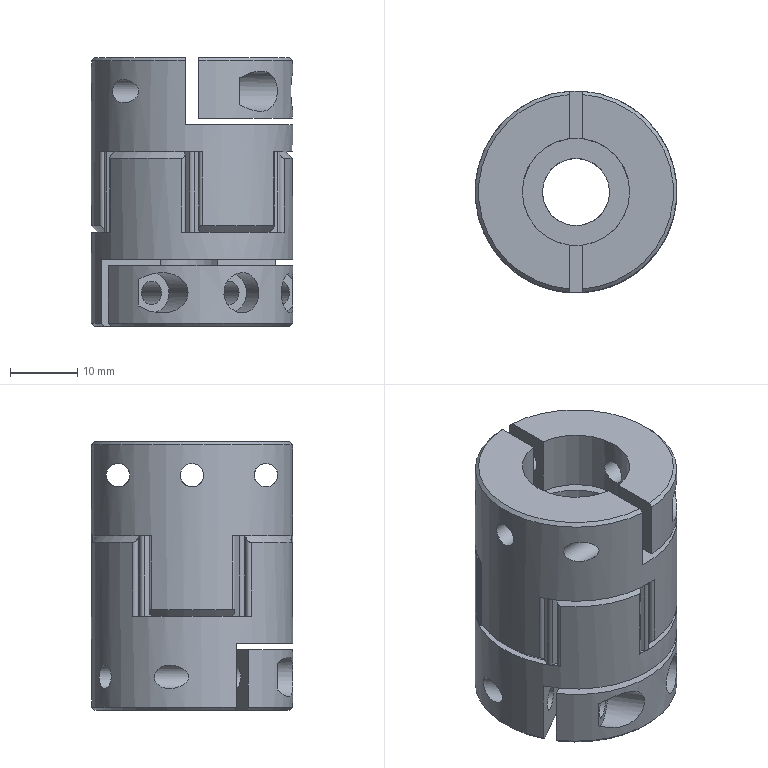Part | STEP file | lianzhou | 5 solids | 125 faces | box 30 x 30 x 40 mm | volume 19224 mm3 | cylinder 81 | plane 32 | cone 12 | commonest cylinder face diameters 12 x24 1 x12 3.5 x12 18 x12 1.113 x6 6 x6